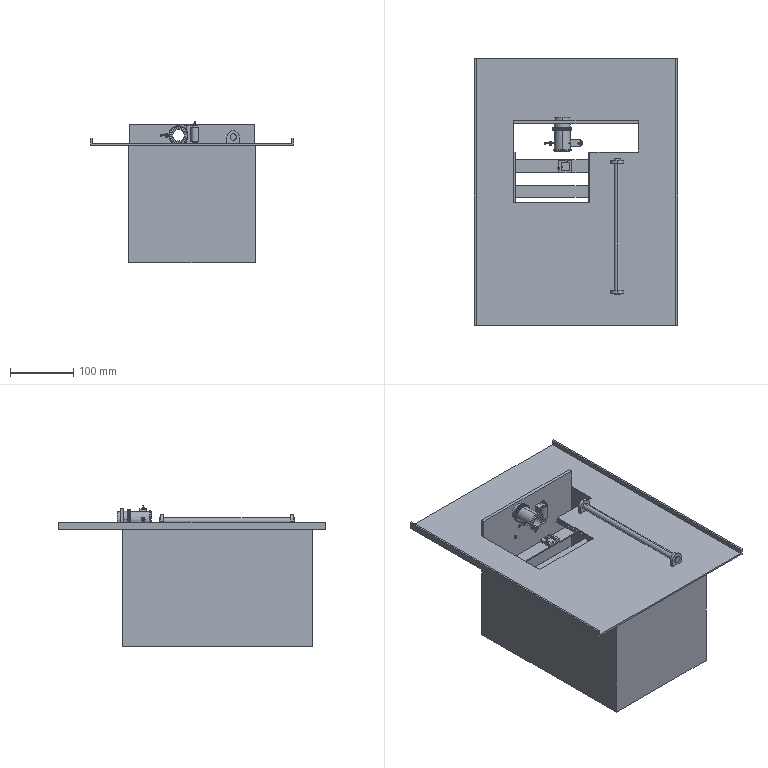Part | SolidWorks | features ICE 27, Cut 8, Fillet 2, BaseBody 1, Chamfer 1, MirrorPattern 1, StudWizard 1 | 10 solids | 536 faces | box 320 x 420 x 222.634 mm | volume 1218802 mm3 | plane 302 | cylinder 224 | cone 8 | torus 2 | commonest cylinder face diameters 28.654 x68 30 x68 2 x14 10 x8 3 x6 6 x6